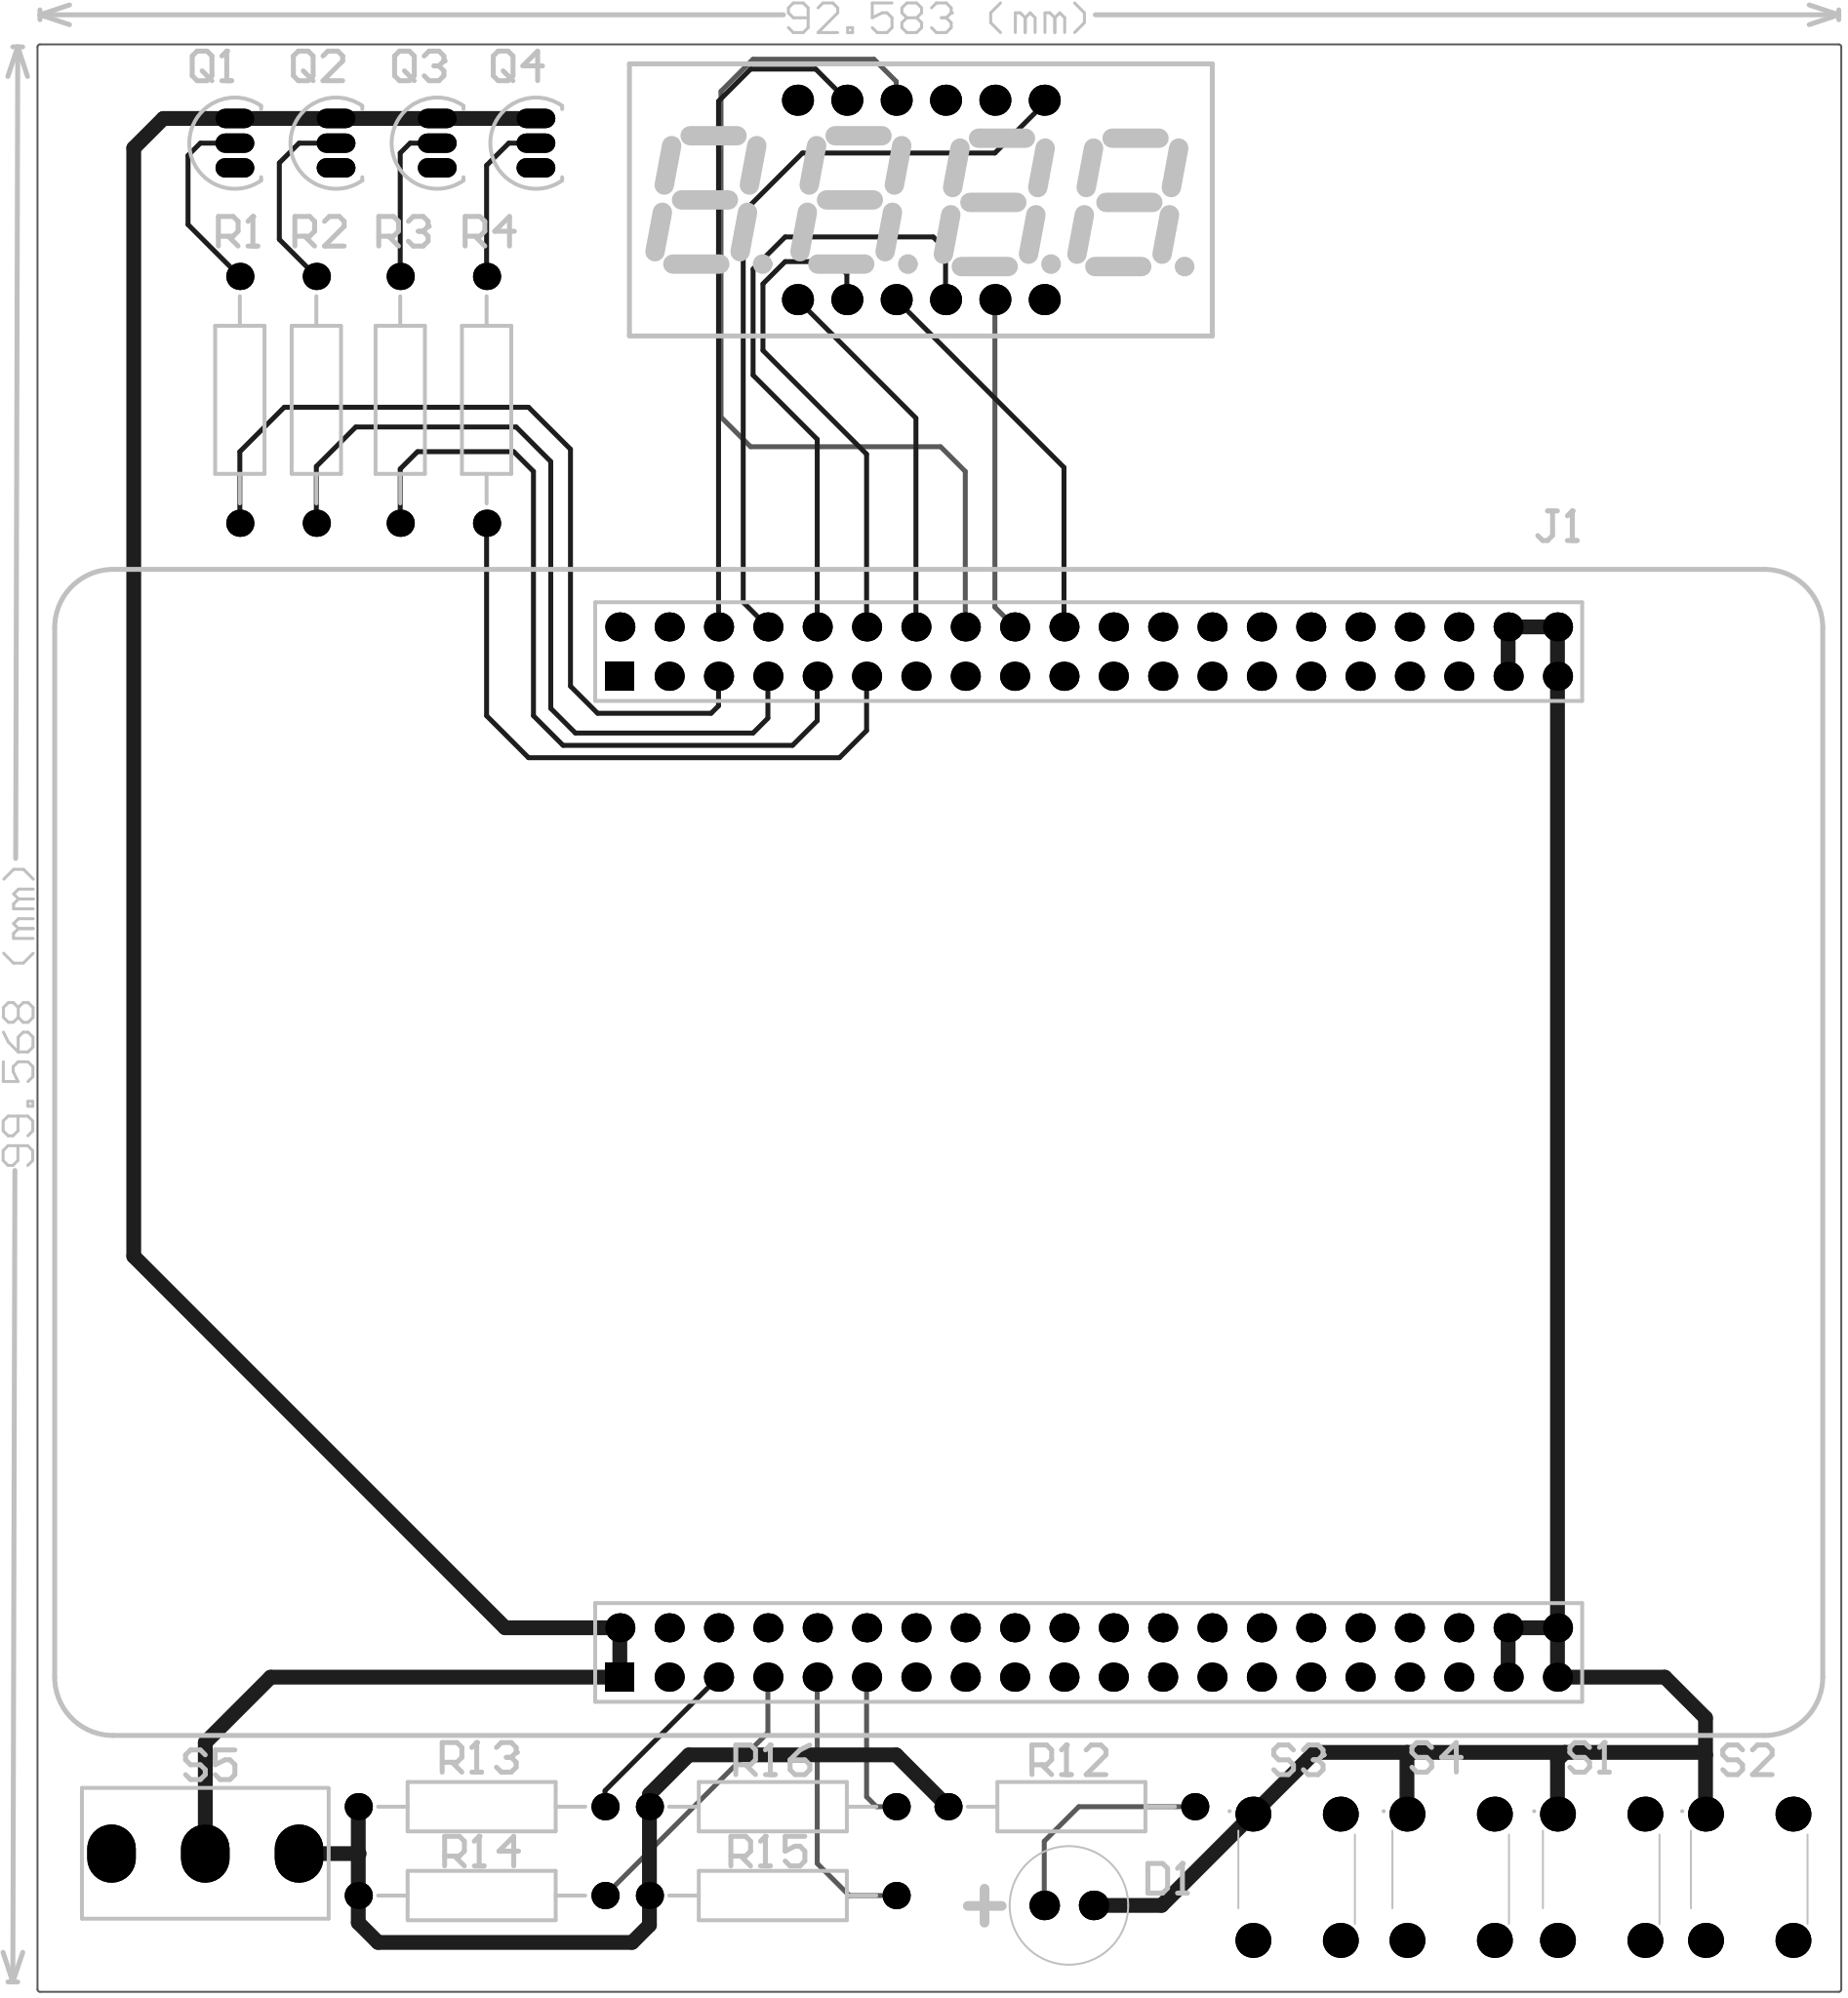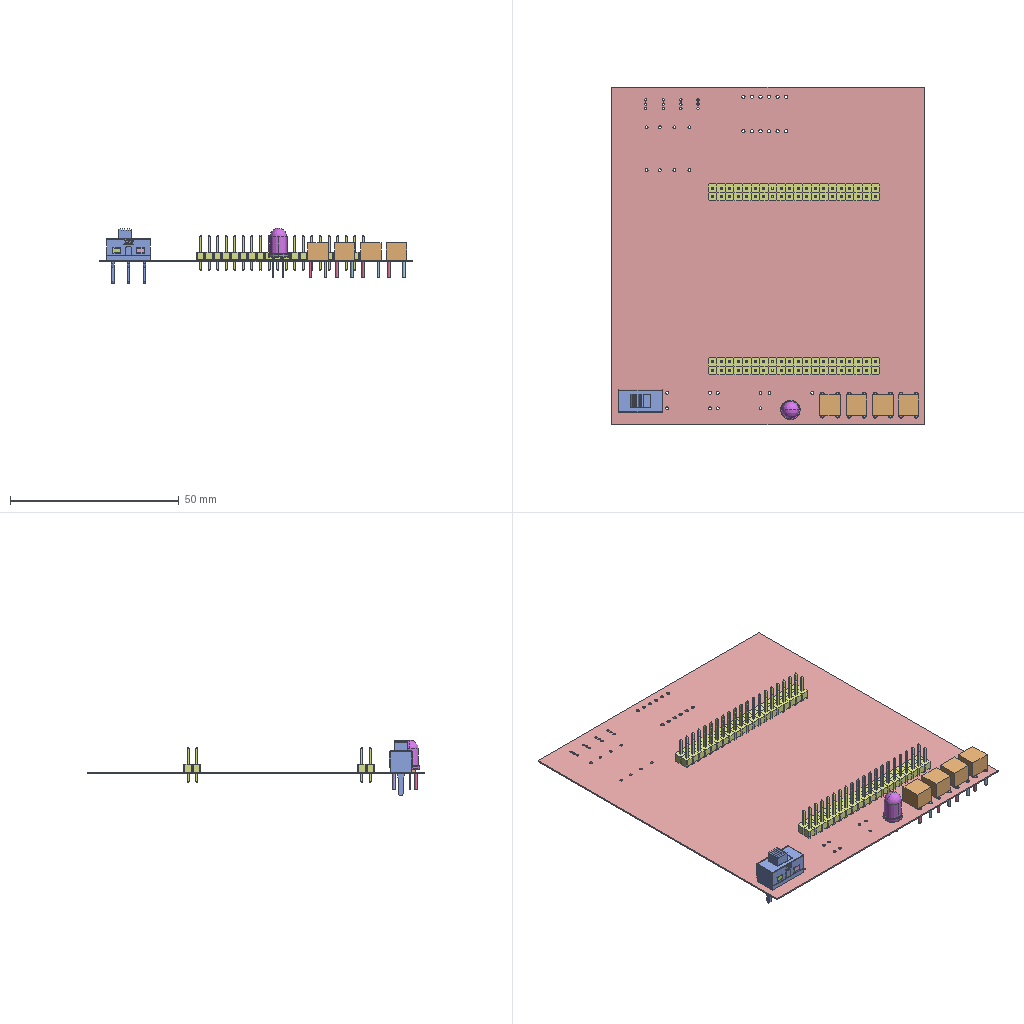Circuit board layout | Altium Designer | box 92.8 x 100.2 x 16.5 mm
Layer stack:
# Altium Designer layer stack of  (unit mm; dielectric type: 0 none, 1 core, 2 prepreg, 3 surface material)
index,name,kind,layer,copper_thickness_mm,dielectric_type,dielectric_thickness_mm,dielectric_material,dielectric_constant
0,Top Paste,other,,,,,,
1,Top Overlay,other,,,,,,
2,Top Solder,dielectric,,,3,0.0102,Solder Resist,3.5
3,Top Layer,copper,Top Layer,0.0356,,,,
4,Dielectric 1,dielectric,,,0,0.32,FR-4,4.8
5,Bottom Layer,copper,Bottom Layer,0.0356,,,,
6,Bottom Solder,dielectric,,,3,0.0102,Solder Resist,3.5
7,Bottom Overlay,other,,,,,,
8,Bottom Paste,other,,,,,,
# drill layer pairs: low layer,high layer
drill_pair,Top Layer,Bottom Layer
Part placement:
Designator,Comment,Layer,Footprint,Center-X(mm),Center-Y(mm),Rotation
,DIG-4,TopLayer,DIG-4,125.349,114.046,360
S5,SW-SPST,TopLayer,SS12D10,88.519,28.956,180
S4,SW-PB,TopLayer,TS665CJ,152.618,27.738,360
S3,SW-PB,TopLayer,TS665CJ,144.689,27.738,360
S2,SW-PB,TopLayer,TS665CJ,167.985,27.738,360
S1,SW-PB,TopLayer,TS665CJ,160.365,27.738,360
R16,Res2,TopLayer,AXIAL-0.5,117.729,31.369,180
R15,Res2,TopLayer,AXIAL-0.5,117.729,26.797,180
R14,Res2,TopLayer,AXIAL-0.5,102.743,26.797,180
R13,Res2,TopLayer,AXIAL-0.5,102.743,31.369,180
R12,Res2,TopLayer,AXIAL-0.5,133.096,31.369,180
R4,,TopLayer,AXIAL-0.5,102.997,103.759,90
R3,,TopLayer,AXIAL-0.5,98.552,103.759,90
R2,,TopLayer,AXIAL-0.5,94.234,103.759,90
R1,,TopLayer,AXIAL-0.5,90.297,103.759,90
Q4,PNP,TopLayer,TO-92,105.537,116.967,360
Q3,PNP,TopLayer,TO-92,100.457,116.967,360
Q2,PNP,TopLayer,TO-92,95.25,116.967,360
Q1,PNP,TopLayer,TO-92,90.043,116.967,360
J1,COREBOARD_CONNECTOR,TopLayer,coreboard_connector,133.985,65.055,360
D1,LED0,TopLayer,LED_TH_HLMP4700,132.969,26.289,360
Pad and via stacks:
# Altium Designer via and pad stacks of  (unit mm). Each distinct definition once, with the count of objects using it.
# via: kind,start_layer,end_layer,hole_mm,diameter_mm,mode(0 simple;1 top-mid-bottom;2 full stack),diameter_per_layer,count,example_net
# pad: kind,layer,hole_mm,hole_type(0 round;1 square;2 slot),plating,top_size,top_shape(1 round;2 rect;3 octagon;9 rounded rect),mid_size,bottom_size,mode,footprint,size_per_layer,count,example
pad,Multi-Layer,0.7,0,plated,2x1,1,2x1,2x1,0,TO-92,,12,Q4.2
pad,Multi-Layer,0.85,0,plated,1.4x1.4,1,1.4x1.4,1.4x1.4,0,AXIAL-0.5,,18,R4.1
pad,Multi-Layer,0.9778,0,plated,1.521x1.521,1,1.521x1.521,1.521x1.521,0,LED_TH_HLMP4700,,2,D1.1
pad,Multi-Layer,0.9,0,plated,1.5x1.5,1,1.5x1.5,1.5x1.5,0,coreboard_connector,,78,J1.40
pad,Multi-Layer,0.9,0,plated,1.5x1.5,2,1.5x1.5,1.5x1.5,0,coreboard_connector,,2,J1.1
pad,Multi-Layer,1.2,0,plated,1.8x1.8,1,1.8x1.8,1.8x1.8,0,TS665CJ,,16,S1.A1
pad,Multi-Layer,1,0,plated,1.6x1.6,1,1.6x1.6,1.6x1.6,0,DIG-4,,12,.1
pad,Multi-Layer,1.2,2,plated,3x2.5,1,3x2.5,3x2.5,0,SS12D10,,3,S5.3
Design rules, without the lines most boards share:
# Altium Designer design rules of  (exported by Altium Designer, unit mm)
# columns: name | kind | enabled | priority | scope1 | scope2 | descriptor | typed fields (field=value)
NetAntennae | 56 | enabled | 1 | All | All | Net Antennae (Tolerance=0mm) (All) |
SilkToSilkClearance | 55 | enabled | 1 | All | All | Silk to Silk (Clearance=0mm) (All),(All) |
SilkToSolderMaskClearance | 54 | enabled | 1 | IsPad | All | Silk To Solder Mask (Clearance=0mm) (IsPad),(All) |
MinimumSolderMaskSliver | 53 | enabled | 1 | All | All | Minimum Solder Mask Sliver (Gap=0mm) (All),(All) |
HoleToHoleClearance | 52 | enabled | 1 | All | All | Hole To Hole Clearance (Gap=0.254mm) (All),(All) | gap=0.254
DiffPairsRouting | 51 | enabled | 1 | All | All | Differential Pairs Uncoupled Length using the Gap Constraints (Min=0.254mm) (Max=0.254mm) (Prefered=0.254mm)  and Width Constraints (Min=0.381mm) (Max=0.381mm) (Prefered=0.381mm) (All) |
HoleSize | 42 | enabled | 1 | All | All | Hole Size Constraint (Min=0.025mm) (Max=2.54mm) (All) |
Height | 50 | enabled | 1 | All | All | Height Constraint (Min=0mm) (Max=25.4mm) (Prefered=12.7mm) (All) | min_height=0 max_height=25.4
ComponentClearance | 24 | enabled | 1 | All | All | Component Clearance Constraint ( Horizontal Gap = 0.254mm, Vertical Gap = 0.254mm ) (All),(All)  | gap=0.254
SolderMaskExpansion | 13 | enabled | 1 | All | All | Solder Mask Expansion (Expansion =0.102mm) (All) | expansion=0.1016
PasteMaskExpansion | 14 | enabled | 1 | All | All | Paste Mask Expansion (Expansion =0mm) (All) | expansion=0
RoutingVias | 11 | enabled | 1 | All | All | Routing Via (MinHoleWidth=0.711mm) (MaxHoleWidth=0.711mm) (PreferredHoleWidth=0.711mm) (MinWidth=1.27mm) (MaxWidth=1.27mm) (PreferedWidth=1.27mm) (All) | via_min_hole=0.7112 via_max_hole=0.7112 via_preferred_diameter=1.27 via_preferred_hole=0.7112
RoutingCorners | 10 | enabled | 1 | All | All | Routing Corners (Style=45-Degree) (Min Setback=2.54mm) (Max Setback=2.54mm) (All) |
Width | 2 | enabled | 1 | All | All | Width Constraint (Min=0.254mm) (Max=0.762mm) (Preferred=0.254mm) (All) |
PolygonConnect | 20 | enabled | 1 | All | All | Polygon Connect Rule(Relief Connect )(Conductor Width=0.254mm) (Relief Angle=90 Angle) (Entries=4) (Air Gap Width=0.254mm) (All),(All) | connect_style(0=relief,1=direct,2=none)=0 relief_conductor_width=0.254 relief_entries=4
PlaneClearance | 12 | enabled | 1 | All | All | Power Plane Clearance (Clearance =0.508mm) (All) | clearance=0.508
PlaneConnect | 6 | enabled | 1 | All | All | Power Plane Connect Rule(Relief Connect )(Expansion=0.508mm) (Conductor Width=0.254mm) (Air Gap=0.254mm) (Entries=4) (All) | relief_conductor_width=0.254 relief_entries=4 relief_expansion=0.508
Clearance | 0 | enabled | 1 | All | All | Clearance Constraint (Gap=0.254mm) (All),(All) | gap=0.254
Classes set for this board:
# Altium Designer classes of  (member kind: 0 net, 1 component, 2 from-to, 3 pad, 4 layer, 5 differential pair, 6 design channel, 7 polygon, 8 structure, 9 xSignal)
# columns: class name | member kind | superclass | members
Sheet2 | 1 | no | D1; J1; Q1; Q2; Q3; Q4; R1; R2; R3; R4; R12; R13; R14; R15; R16; S1; S2; S3; S4; S5;